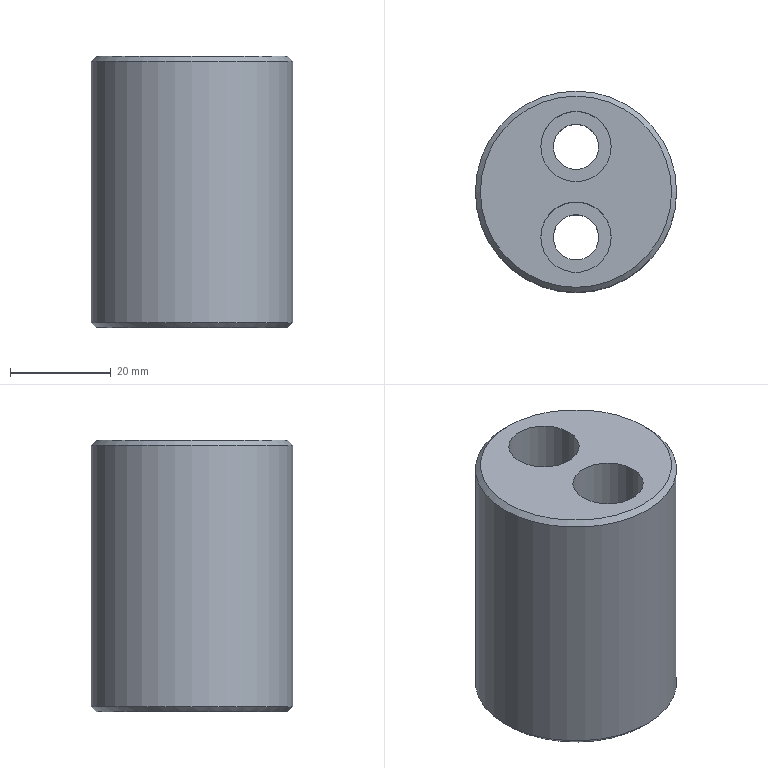Part | NX | features solid 2 | 1 solid | 11 faces | box 40 x 40 x 54 mm | volume 53819 mm3 | cylinder 5 | plane 4 | cone 2 | commonest cylinder face diameters 9 x2 14 x2 40 x1
STEP:
#1=CARTESIAN_POINT('',(331.,84.,65.));
#2=VERTEX_POINT('',#1);
#3=CARTESIAN_POINT('',(326.5,84.,65.));
#4=DIRECTION('',(0.,0.,1.));
#5=DIRECTION('',(1.,0.,0.));
#6=AXIS2_PLACEMENT_3D('',#3,#4,#5);
#7=CIRCLE('',#6,4.5);
#8=EDGE_CURVE('',#2,#2,#7,.F.);
#9=ORIENTED_EDGE('',*,*,#8,.T.);
#10=EDGE_LOOP('',(#9));
#11=FACE_BOUND('',#10,.T.);
#12=CARTESIAN_POINT('',(333.5,84.,65.));
#13=VERTEX_POINT('',#12);
#14=CARTESIAN_POINT('',(326.5,84.,65.));
#15=DIRECTION('',(0.,0.,1.));
#16=DIRECTION('',(1.,0.,0.));
#17=AXIS2_PLACEMENT_3D('',#14,#15,#16);
#18=CIRCLE('',#17,7.);
#19=EDGE_CURVE('',#13,#13,#18,.F.);
#20=ORIENTED_EDGE('',*,*,#19,.F.);
#21=EDGE_LOOP('',(#20));
#22=FACE_BOUND('',#21,.T.);
#23=CARTESIAN_POINT('',(500.879,-61.,65.));
#24=DIRECTION('',(0.,0.,1.));
#25=DIRECTION('',(1.,0.,0.));
#26=AXIS2_PLACEMENT_3D('',#23,#24,#25);
#27=PLANE('',#26);
#28=ADVANCED_FACE('',(#11,#22),#27,.T.);
#29=ORIENTED_EDGE('',*,*,#8,.F.);
#30=EDGE_LOOP('',(#29));
#31=FACE_BOUND('',#30,.T.);
#32=CARTESIAN_POINT('',(331.,84.,50.));
#33=VERTEX_POINT('',#32);
#34=CARTESIAN_POINT('',(326.5,84.,50.));
#35=DIRECTION('',(0.,0.,1.));
#36=DIRECTION('',(1.,0.,0.));
#37=AXIS2_PLACEMENT_3D('',#34,#35,#36);
#38=CIRCLE('',#37,4.5);
#39=EDGE_CURVE('',#33,#33,#38,.F.);
#40=ORIENTED_EDGE('',*,*,#39,.T.);
#41=EDGE_LOOP('',(#40));
#42=FACE_BOUND('',#41,.T.);
#43=CARTESIAN_POINT('',(326.5,84.,45.));
#44=DIRECTION('',(0.,0.,-1.));
#45=DIRECTION('',(-1.,0.,0.));
#46=AXIS2_PLACEMENT_3D('',#43,#44,#45);
#47=CYLINDRICAL_SURFACE('',#46,4.5);
#48=ADVANCED_FACE('',(#31,#42),#47,.F.);
#49=ORIENTED_EDGE('',*,*,#19,.T.);
#50=EDGE_LOOP('',(#49));
#51=FACE_BOUND('',#50,.T.);
#52=CARTESIAN_POINT('',(333.5,84.,104.));
#53=VERTEX_POINT('',#52);
#54=CARTESIAN_POINT('',(326.5,84.,104.));
#55=DIRECTION('',(0.,0.,-1.));
#56=DIRECTION('',(1.,0.,0.));
#57=AXIS2_PLACEMENT_3D('',#54,#55,#56);
#58=CIRCLE('',#57,7.);
#59=EDGE_CURVE('',#53,#53,#58,.F.);
#60=ORIENTED_EDGE('',*,*,#59,.T.);
#61=EDGE_LOOP('',(#60));
#62=FACE_BOUND('',#61,.T.);
#63=CARTESIAN_POINT('',(326.5,84.,70.));
#64=DIRECTION('',(0.,0.,-1.));
#65=DIRECTION('',(-1.,0.,0.));
#66=AXIS2_PLACEMENT_3D('',#63,#64,#65);
#67=CYLINDRICAL_SURFACE('',#66,7.);
#68=ADVANCED_FACE('',(#51,#62),#67,.F.);
#69=CARTESIAN_POINT('',(346.5,93.,51.));
#70=VERTEX_POINT('',#69);
#71=CARTESIAN_POINT('',(326.5,93.,51.));
#72=DIRECTION('',(0.,0.,-1.));
#73=DIRECTION('',(1.,0.,0.));
#74=AXIS2_PLACEMENT_3D('',#71,#72,#73);
#75=CIRCLE('',#74,20.);
#76=EDGE_CURVE('',#70,#70,#75,.T.);
#77=ORIENTED_EDGE('',*,*,#76,.F.);
#78=EDGE_LOOP('',(#77));
#79=FACE_BOUND('',#78,.T.);
#80=CARTESIAN_POINT('',(306.5,93.,103.));
#81=VERTEX_POINT('',#80);
#82=CARTESIAN_POINT('',(326.5,93.,103.));
#83=DIRECTION('',(0.,0.,1.));
#84=DIRECTION('',(-1.,0.,0.));
#85=AXIS2_PLACEMENT_3D('',#82,#83,#84);
#86=CIRCLE('',#85,20.);
#87=EDGE_CURVE('',#81,#81,#86,.T.);
#88=ORIENTED_EDGE('',*,*,#87,.F.);
#89=EDGE_LOOP('',(#88));
#90=FACE_BOUND('',#89,.T.);
#91=CARTESIAN_POINT('',(326.5,93.,58.));
#92=DIRECTION('',(0.,0.,-1.));
#93=DIRECTION('',(-1.,0.,0.));
#94=AXIS2_PLACEMENT_3D('',#91,#92,#93);
#95=CYLINDRICAL_SURFACE('',#94,20.);
#96=ADVANCED_FACE('',(#79,#90),#95,.T.);
#97=CARTESIAN_POINT('',(331.,102.,65.));
#98=VERTEX_POINT('',#97);
#99=CARTESIAN_POINT('',(326.5,102.,65.));
#100=DIRECTION('',(0.,0.,-1.));
#101=DIRECTION('',(1.,0.,0.));
#102=AXIS2_PLACEMENT_3D('',#99,#100,#101);
#103=CIRCLE('',#102,4.5);
#104=EDGE_CURVE('',#98,#98,#103,.T.);
#105=ORIENTED_EDGE('',*,*,#104,.T.);
#106=EDGE_LOOP('',(#105));
#107=FACE_BOUND('',#106,.T.);
#108=CARTESIAN_POINT('',(333.5,102.,65.));
#109=VERTEX_POINT('',#108);
#110=CARTESIAN_POINT('',(326.5,102.,65.));
#111=DIRECTION('',(0.,0.,-1.));
#112=DIRECTION('',(1.,0.,0.));
#113=AXIS2_PLACEMENT_3D('',#110,#111,#112);
#114=CIRCLE('',#113,7.);
#115=EDGE_CURVE('',#109,#109,#114,.T.);
#116=ORIENTED_EDGE('',*,*,#115,.F.);
#117=EDGE_LOOP('',(#116));
#118=FACE_BOUND('',#117,.T.);
#119=CARTESIAN_POINT('',(500.879,247.,65.));
#120=DIRECTION('',(0.,0.,1.));
#121=DIRECTION('',(1.,0.,0.));
#122=AXIS2_PLACEMENT_3D('',#119,#120,#121);
#123=PLANE('',#122);
#124=ADVANCED_FACE('',(#107,#118),#123,.T.);
#125=CARTESIAN_POINT('',(345.5,93.,50.));
#126=VERTEX_POINT('',#125);
#127=CARTESIAN_POINT('',(326.5,93.,50.));
#128=DIRECTION('',(0.,0.,-1.));
#129=DIRECTION('',(1.,0.,0.));
#130=AXIS2_PLACEMENT_3D('',#127,#128,#129);
#131=CIRCLE('',#130,19.);
#132=EDGE_CURVE('',#126,#126,#131,.F.);
#133=ORIENTED_EDGE('',*,*,#132,.T.);
#134=EDGE_LOOP('',(#133));
#135=FACE_BOUND('',#134,.T.);
#136=ORIENTED_EDGE('',*,*,#76,.T.);
#137=EDGE_LOOP('',(#136));
#138=FACE_BOUND('',#137,.T.);
#139=CARTESIAN_POINT('',(326.5,93.,51.));
#140=DIRECTION('',(0.,0.,1.));
#141=DIRECTION('',(1.,0.,0.));
#142=AXIS2_PLACEMENT_3D('',#139,#140,#141);
#143=CONICAL_SURFACE('',#142,20.,0.7854);
#144=ADVANCED_FACE('',(#135,#138),#143,.T.);
#145=ORIENTED_EDGE('',*,*,#104,.F.);
#146=EDGE_LOOP('',(#145));
#147=FACE_BOUND('',#146,.T.);
#148=CARTESIAN_POINT('',(331.,102.,50.));
#149=VERTEX_POINT('',#148);
#150=CARTESIAN_POINT('',(326.5,102.,50.));
#151=DIRECTION('',(0.,0.,-1.));
#152=DIRECTION('',(1.,0.,0.));
#153=AXIS2_PLACEMENT_3D('',#150,#151,#152);
#154=CIRCLE('',#153,4.5);
#155=EDGE_CURVE('',#149,#149,#154,.T.);
#156=ORIENTED_EDGE('',*,*,#155,.T.);
#157=EDGE_LOOP('',(#156));
#158=FACE_BOUND('',#157,.T.);
#159=CARTESIAN_POINT('',(326.5,102.,45.));
#160=DIRECTION('',(0.,0.,-1.));
#161=DIRECTION('',(-1.,0.,0.));
#162=AXIS2_PLACEMENT_3D('',#159,#160,#161);
#163=CYLINDRICAL_SURFACE('',#162,4.5);
#164=ADVANCED_FACE('',(#147,#158),#163,.F.);
#165=ORIENTED_EDGE('',*,*,#39,.F.);
#166=EDGE_LOOP('',(#165));
#167=FACE_BOUND('',#166,.T.);
#168=ORIENTED_EDGE('',*,*,#155,.F.);
#169=EDGE_LOOP('',(#168));
#170=FACE_BOUND('',#169,.T.);
#171=ORIENTED_EDGE('',*,*,#132,.F.);
#172=EDGE_LOOP('',(#171));
#173=FACE_BOUND('',#172,.T.);
#174=CARTESIAN_POINT('',(500.879,238.,50.));
#175=DIRECTION('',(0.,0.,1.));
#176=DIRECTION('',(1.,0.,0.));
#177=AXIS2_PLACEMENT_3D('',#174,#175,#176);
#178=PLANE('',#177);
#179=ADVANCED_FACE('',(#167,#170,#173),#178,.F.);
#180=ORIENTED_EDGE('',*,*,#87,.T.);
#181=EDGE_LOOP('',(#180));
#182=FACE_BOUND('',#181,.T.);
#183=CARTESIAN_POINT('',(345.5,93.,104.));
#184=VERTEX_POINT('',#183);
#185=CARTESIAN_POINT('',(326.5,93.,104.));
#186=DIRECTION('',(0.,0.,-1.));
#187=DIRECTION('',(1.,0.,0.));
#188=AXIS2_PLACEMENT_3D('',#185,#186,#187);
#189=CIRCLE('',#188,19.);
#190=EDGE_CURVE('',#184,#184,#189,.T.);
#191=ORIENTED_EDGE('',*,*,#190,.T.);
#192=EDGE_LOOP('',(#191));
#193=FACE_BOUND('',#192,.T.);
#194=CARTESIAN_POINT('',(326.5,93.,104.));
#195=DIRECTION('',(0.,0.,-1.));
#196=DIRECTION('',(-1.,0.,0.));
#197=AXIS2_PLACEMENT_3D('',#194,#195,#196);
#198=CONICAL_SURFACE('',#197,19.,0.7854);
#199=ADVANCED_FACE('',(#182,#193),#198,.T.);
#200=ORIENTED_EDGE('',*,*,#115,.T.);
#201=EDGE_LOOP('',(#200));
#202=FACE_BOUND('',#201,.T.);
#203=CARTESIAN_POINT('',(333.5,102.,104.));
#204=VERTEX_POINT('',#203);
#205=CARTESIAN_POINT('',(326.5,102.,104.));
#206=DIRECTION('',(0.,0.,-1.));
#207=DIRECTION('',(1.,0.,0.));
#208=AXIS2_PLACEMENT_3D('',#205,#206,#207);
#209=CIRCLE('',#208,7.);
#210=EDGE_CURVE('',#204,#204,#209,.F.);
#211=ORIENTED_EDGE('',*,*,#210,.T.);
#212=EDGE_LOOP('',(#211));
#213=FACE_BOUND('',#212,.T.);
#214=CARTESIAN_POINT('',(326.5,102.,70.));
#215=DIRECTION('',(0.,0.,-1.));
#216=DIRECTION('',(-1.,0.,0.));
#217=AXIS2_PLACEMENT_3D('',#214,#215,#216);
#218=CYLINDRICAL_SURFACE('',#217,7.);
#219=ADVANCED_FACE('',(#202,#213),#218,.F.);
#220=ORIENTED_EDGE('',*,*,#59,.F.);
#221=EDGE_LOOP('',(#220));
#222=FACE_BOUND('',#221,.T.);
#223=ORIENTED_EDGE('',*,*,#210,.F.);
#224=EDGE_LOOP('',(#223));
#225=FACE_BOUND('',#224,.T.);
#226=ORIENTED_EDGE('',*,*,#190,.F.);
#227=EDGE_LOOP('',(#226));
#228=FACE_BOUND('',#227,.T.);
#229=CARTESIAN_POINT('',(326.5,-7.,104.));
#230=DIRECTION('',(0.,0.,1.));
#231=DIRECTION('',(-1.,0.,0.));
#232=AXIS2_PLACEMENT_3D('',#229,#230,#231);
#233=PLANE('',#232);
#234=ADVANCED_FACE('',(#222,#225,#228),#233,.T.);
#235=CLOSED_SHELL('',(#28,#48,#68,#96,#124,#144,#164,#179,#199,#219,#234));
#236=MANIFOLD_SOLID_BREP('',#235);
#237=(LENGTH_UNIT()NAMED_UNIT(*)SI_UNIT(.MILLI.,.METRE.));
#238=UNCERTAINTY_MEASURE_WITH_UNIT(LENGTH_MEASURE(0.00001),#237,'','');
#239=(NAMED_UNIT(*)PLANE_ANGLE_UNIT()SI_UNIT($,.RADIAN.));
#240=(NAMED_UNIT(*)SI_UNIT($,.STERADIAN.)SOLID_ANGLE_UNIT());
#241=(GEOMETRIC_REPRESENTATION_CONTEXT(3)GLOBAL_UNCERTAINTY_ASSIGNED_CONTEXT((#238))GLOBAL_UNIT_ASSIGNED_CONTEXT((#237,#239,#240))REPRESENTATION_CONTEXT('',''));
#242=ADVANCED_BREP_SHAPE_REPRESENTATION('',(#236),#241);